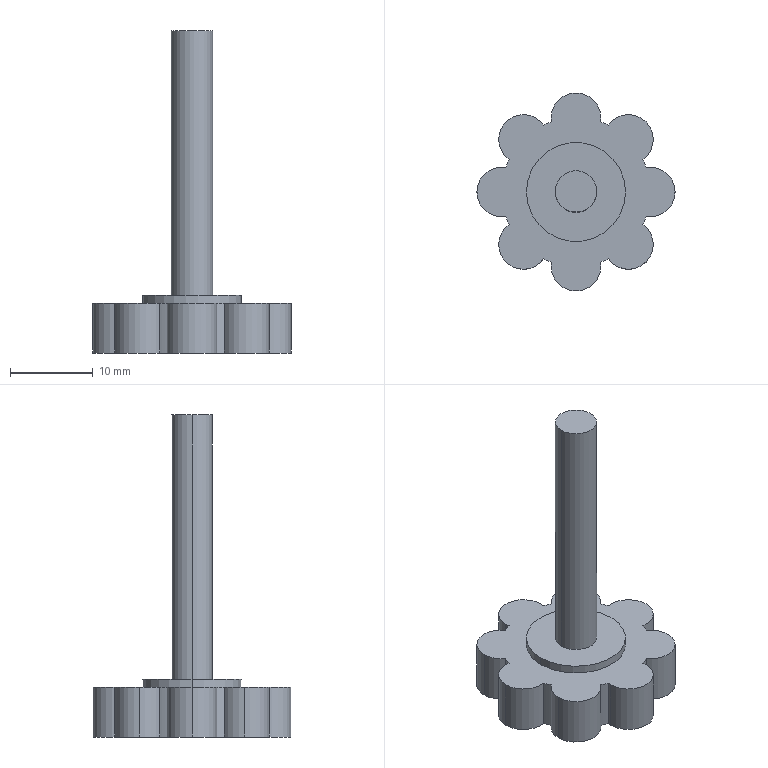Part | SolidWorks | features ICE 3, Extrusion 1 | 1 solid | 34 faces | box 24 x 24 x 39 mm | volume 2986 mm3 | cylinder 29 | plane 5 | commonest cylinder face diameters 6 x15 18 x8 5 x2 7.409 x2 12 x2
STEP:
#1=CARTESIAN_POINT('',(3.705,0.,0.2));
#2=VERTEX_POINT('',#1);
#3=CARTESIAN_POINT('',(-3.705,0.,0.2));
#4=VERTEX_POINT('',#3);
#5=CARTESIAN_POINT('',(0.,0.,0.2));
#6=DIRECTION('',(0.,0.,-1.));
#7=DIRECTION('',(-1.,0.,0.));
#8=AXIS2_PLACEMENT_3D('',#5,#6,#7);
#9=CIRCLE('',#8,3.705);
#10=EDGE_CURVE('',#2,#4,#9,.T.);
#11=ORIENTED_EDGE('',*,*,#10,.F.);
#12=CARTESIAN_POINT('',(3.705,0.,0.));
#13=VERTEX_POINT('',#12);
#14=CARTESIAN_POINT('',(3.705,0.,0.2));
#15=DIRECTION('',(0.,0.,-1.));
#16=VECTOR('',#15,1000.);
#17=LINE('',#14,#16);
#18=EDGE_CURVE('',#2,#13,#17,.T.);
#19=ORIENTED_EDGE('',*,*,#18,.T.);
#20=CARTESIAN_POINT('',(-3.705,0.,0.));
#21=VERTEX_POINT('',#20);
#22=CARTESIAN_POINT('',(0.,0.,0.));
#23=DIRECTION('',(0.,0.,-1.));
#24=DIRECTION('',(-1.,0.,0.));
#25=AXIS2_PLACEMENT_3D('',#22,#23,#24);
#26=CIRCLE('',#25,3.705);
#27=EDGE_CURVE('',#13,#21,#26,.T.);
#28=ORIENTED_EDGE('',*,*,#27,.T.);
#29=CARTESIAN_POINT('',(-3.705,0.,0.2));
#30=DIRECTION('',(0.,0.,-1.));
#31=VECTOR('',#30,1000.);
#32=LINE('',#29,#31);
#33=EDGE_CURVE('',#4,#21,#32,.T.);
#34=ORIENTED_EDGE('',*,*,#33,.F.);
#35=EDGE_LOOP('',(#11,#19,#28,#34));
#36=FACE_OUTER_BOUND('',#35,.T.);
#37=CARTESIAN_POINT('',(0.,0.,0.2));
#38=DIRECTION('',(0.,0.,-1.));
#39=DIRECTION('',(-1.,0.,0.));
#40=AXIS2_PLACEMENT_3D('',#37,#38,#39);
#41=CYLINDRICAL_SURFACE('',#40,3.705);
#42=ADVANCED_FACE('',(#36),#41,.F.);
#43=CARTESIAN_POINT('',(2.5,0.,39.));
#44=VERTEX_POINT('',#43);
#45=CARTESIAN_POINT('',(-2.5,0.,39.));
#46=VERTEX_POINT('',#45);
#47=CARTESIAN_POINT('',(0.,0.,39.));
#48=DIRECTION('',(0.,0.,1.));
#49=DIRECTION('',(1.,0.,0.));
#50=AXIS2_PLACEMENT_3D('',#47,#48,#49);
#51=CIRCLE('',#50,2.5);
#52=EDGE_CURVE('',#44,#46,#51,.T.);
#53=ORIENTED_EDGE('',*,*,#52,.F.);
#54=CARTESIAN_POINT('',(2.5,0.,7.));
#55=VERTEX_POINT('',#54);
#56=CARTESIAN_POINT('',(2.5,0.,39.));
#57=DIRECTION('',(0.,0.,-1.));
#58=VECTOR('',#57,1000.);
#59=LINE('',#56,#58);
#60=EDGE_CURVE('',#44,#55,#59,.T.);
#61=ORIENTED_EDGE('',*,*,#60,.T.);
#62=CARTESIAN_POINT('',(-2.5,0.,7.));
#63=VERTEX_POINT('',#62);
#64=CARTESIAN_POINT('',(0.,0.,7.));
#65=DIRECTION('',(0.,0.,1.));
#66=DIRECTION('',(1.,0.,0.));
#67=AXIS2_PLACEMENT_3D('',#64,#65,#66);
#68=CIRCLE('',#67,2.5);
#69=EDGE_CURVE('',#55,#63,#68,.T.);
#70=ORIENTED_EDGE('',*,*,#69,.T.);
#71=CARTESIAN_POINT('',(-2.5,0.,39.));
#72=DIRECTION('',(0.,0.,-1.));
#73=VECTOR('',#72,1000.);
#74=LINE('',#71,#73);
#75=EDGE_CURVE('',#46,#63,#74,.T.);
#76=ORIENTED_EDGE('',*,*,#75,.F.);
#77=EDGE_LOOP('',(#53,#61,#70,#76));
#78=FACE_OUTER_BOUND('',#77,.T.);
#79=CARTESIAN_POINT('',(0.,0.,39.));
#80=DIRECTION('',(0.,0.,-1.));
#81=DIRECTION('',(-1.,0.,0.));
#82=AXIS2_PLACEMENT_3D('',#79,#80,#81);
#83=CYLINDRICAL_SURFACE('',#82,2.5);
#84=ADVANCED_FACE('',(#78),#83,.T.);
#85=CARTESIAN_POINT('',(6.,0.,7.));
#86=VERTEX_POINT('',#85);
#87=CARTESIAN_POINT('',(-6.,0.,7.));
#88=VERTEX_POINT('',#87);
#89=CARTESIAN_POINT('',(0.,0.,7.));
#90=DIRECTION('',(0.,0.,1.));
#91=DIRECTION('',(1.,0.,0.));
#92=AXIS2_PLACEMENT_3D('',#89,#90,#91);
#93=CIRCLE('',#92,6.);
#94=EDGE_CURVE('',#86,#88,#93,.T.);
#95=ORIENTED_EDGE('',*,*,#94,.F.);
#96=CARTESIAN_POINT('',(6.,0.,6.));
#97=VERTEX_POINT('',#96);
#98=CARTESIAN_POINT('',(6.,0.,7.));
#99=DIRECTION('',(0.,0.,-1.));
#100=VECTOR('',#99,1000.);
#101=LINE('',#98,#100);
#102=EDGE_CURVE('',#86,#97,#101,.T.);
#103=ORIENTED_EDGE('',*,*,#102,.T.);
#104=CARTESIAN_POINT('',(-6.,0.,6.));
#105=VERTEX_POINT('',#104);
#106=CARTESIAN_POINT('',(0.,0.,6.));
#107=DIRECTION('',(0.,0.,-1.));
#108=DIRECTION('',(1.,0.,0.));
#109=AXIS2_PLACEMENT_3D('',#106,#107,#108);
#110=CIRCLE('',#109,6.);
#111=EDGE_CURVE('',#105,#97,#110,.T.);
#112=ORIENTED_EDGE('',*,*,#111,.F.);
#113=CARTESIAN_POINT('',(-6.,0.,7.));
#114=DIRECTION('',(0.,0.,-1.));
#115=VECTOR('',#114,1000.);
#116=LINE('',#113,#115);
#117=EDGE_CURVE('',#88,#105,#116,.T.);
#118=ORIENTED_EDGE('',*,*,#117,.F.);
#119=EDGE_LOOP('',(#95,#103,#112,#118));
#120=FACE_OUTER_BOUND('',#119,.T.);
#121=CARTESIAN_POINT('',(0.,0.,7.));
#122=DIRECTION('',(0.,0.,-1.));
#123=DIRECTION('',(-1.,0.,0.));
#124=AXIS2_PLACEMENT_3D('',#121,#122,#123);
#125=CYLINDRICAL_SURFACE('',#124,6.);
#126=ADVANCED_FACE('',(#120),#125,.T.);
#127=CARTESIAN_POINT('',(-9.364,6.364,6.));
#128=VERTEX_POINT('',#127);
#129=CARTESIAN_POINT('',(-8.102,3.919,6.));
#130=VERTEX_POINT('',#129);
#131=CARTESIAN_POINT('',(-6.364,6.364,6.));
#132=DIRECTION('',(0.,0.,1.));
#133=DIRECTION('',(1.,0.,0.));
#134=AXIS2_PLACEMENT_3D('',#131,#132,#133);
#135=CIRCLE('',#134,3.);
#136=EDGE_CURVE('',#128,#130,#135,.T.);
#137=ORIENTED_EDGE('',*,*,#136,.F.);
#138=CARTESIAN_POINT('',(-9.364,6.364,0.));
#139=VERTEX_POINT('',#138);
#140=CARTESIAN_POINT('',(-9.364,6.364,6.));
#141=DIRECTION('',(0.,0.,-1.));
#142=VECTOR('',#141,1000.);
#143=LINE('',#140,#142);
#144=EDGE_CURVE('',#128,#139,#143,.T.);
#145=ORIENTED_EDGE('',*,*,#144,.T.);
#146=CARTESIAN_POINT('',(-8.102,3.919,0.));
#147=VERTEX_POINT('',#146);
#148=CARTESIAN_POINT('',(-6.364,6.364,0.));
#149=DIRECTION('',(0.,0.,1.));
#150=DIRECTION('',(1.,0.,0.));
#151=AXIS2_PLACEMENT_3D('',#148,#149,#150);
#152=CIRCLE('',#151,3.);
#153=EDGE_CURVE('',#139,#147,#152,.T.);
#154=ORIENTED_EDGE('',*,*,#153,.T.);
#155=CARTESIAN_POINT('',(-8.102,3.919,6.));
#156=DIRECTION('',(0.,0.,-1.));
#157=VECTOR('',#156,1000.);
#158=LINE('',#155,#157);
#159=EDGE_CURVE('',#130,#147,#158,.T.);
#160=ORIENTED_EDGE('',*,*,#159,.F.);
#161=EDGE_LOOP('',(#137,#145,#154,#160));
#162=FACE_OUTER_BOUND('',#161,.T.);
#163=CARTESIAN_POINT('',(-6.364,6.364,6.));
#164=DIRECTION('',(0.,0.,-1.));
#165=DIRECTION('',(-1.,0.,0.));
#166=AXIS2_PLACEMENT_3D('',#163,#164,#165);
#167=CYLINDRICAL_SURFACE('',#166,3.);
#168=ADVANCED_FACE('',(#162),#167,.T.);
#169=CARTESIAN_POINT('',(3.,9.,6.));
#170=VERTEX_POINT('',#169);
#171=CARTESIAN_POINT('',(-3.,9.,6.));
#172=VERTEX_POINT('',#171);
#173=CARTESIAN_POINT('',(0.,9.,6.));
#174=DIRECTION('',(0.,0.,1.));
#175=DIRECTION('',(1.,0.,0.));
#176=AXIS2_PLACEMENT_3D('',#173,#174,#175);
#177=CIRCLE('',#176,3.);
#178=EDGE_CURVE('',#170,#172,#177,.T.);
#179=ORIENTED_EDGE('',*,*,#178,.F.);
#180=CARTESIAN_POINT('',(3.,9.,0.));
#181=VERTEX_POINT('',#180);
#182=CARTESIAN_POINT('',(3.,9.,6.));
#183=DIRECTION('',(0.,0.,-1.));
#184=VECTOR('',#183,1000.);
#185=LINE('',#182,#184);
#186=EDGE_CURVE('',#170,#181,#185,.T.);
#187=ORIENTED_EDGE('',*,*,#186,.T.);
#188=CARTESIAN_POINT('',(-3.,9.,0.));
#189=VERTEX_POINT('',#188);
#190=CARTESIAN_POINT('',(0.,9.,0.));
#191=DIRECTION('',(0.,0.,1.));
#192=DIRECTION('',(1.,0.,0.));
#193=AXIS2_PLACEMENT_3D('',#190,#191,#192);
#194=CIRCLE('',#193,3.);
#195=EDGE_CURVE('',#181,#189,#194,.T.);
#196=ORIENTED_EDGE('',*,*,#195,.T.);
#197=CARTESIAN_POINT('',(-3.,9.,6.));
#198=DIRECTION('',(0.,0.,-1.));
#199=VECTOR('',#198,1000.);
#200=LINE('',#197,#199);
#201=EDGE_CURVE('',#172,#189,#200,.T.);
#202=ORIENTED_EDGE('',*,*,#201,.F.);
#203=EDGE_LOOP('',(#179,#187,#196,#202));
#204=FACE_OUTER_BOUND('',#203,.T.);
#205=CARTESIAN_POINT('',(0.,9.,6.));
#206=DIRECTION('',(0.,0.,-1.));
#207=DIRECTION('',(-1.,0.,0.));
#208=AXIS2_PLACEMENT_3D('',#205,#206,#207);
#209=CYLINDRICAL_SURFACE('',#208,3.);
#210=ADVANCED_FACE('',(#204),#209,.T.);
#211=CARTESIAN_POINT('',(-2.958,8.5,6.));
#212=VERTEX_POINT('',#211);
#213=CARTESIAN_POINT('',(0.,9.,6.));
#214=DIRECTION('',(0.,0.,1.));
#215=DIRECTION('',(1.,0.,0.));
#216=AXIS2_PLACEMENT_3D('',#213,#214,#215);
#217=CIRCLE('',#216,3.);
#218=EDGE_CURVE('',#172,#212,#217,.T.);
#219=ORIENTED_EDGE('',*,*,#218,.F.);
#220=ORIENTED_EDGE('',*,*,#201,.T.);
#221=CARTESIAN_POINT('',(-2.958,8.5,0.));
#222=VERTEX_POINT('',#221);
#223=CARTESIAN_POINT('',(0.,9.,0.));
#224=DIRECTION('',(0.,0.,1.));
#225=DIRECTION('',(1.,0.,0.));
#226=AXIS2_PLACEMENT_3D('',#223,#224,#225);
#227=CIRCLE('',#226,3.);
#228=EDGE_CURVE('',#189,#222,#227,.T.);
#229=ORIENTED_EDGE('',*,*,#228,.T.);
#230=CARTESIAN_POINT('',(-2.958,8.5,6.));
#231=DIRECTION('',(0.,0.,-1.));
#232=VECTOR('',#231,1000.);
#233=LINE('',#230,#232);
#234=EDGE_CURVE('',#212,#222,#233,.T.);
#235=ORIENTED_EDGE('',*,*,#234,.F.);
#236=EDGE_LOOP('',(#219,#220,#229,#235));
#237=FACE_OUTER_BOUND('',#236,.T.);
#238=CARTESIAN_POINT('',(0.,9.,6.));
#239=DIRECTION('',(0.,0.,-1.));
#240=DIRECTION('',(-1.,0.,0.));
#241=AXIS2_PLACEMENT_3D('',#238,#239,#240);
#242=CYLINDRICAL_SURFACE('',#241,3.);
#243=ADVANCED_FACE('',(#237),#242,.T.);
#244=CARTESIAN_POINT('',(3.,-9.,6.));
#245=VERTEX_POINT('',#244);
#246=CARTESIAN_POINT('',(2.958,-8.5,6.));
#247=VERTEX_POINT('',#246);
#248=CARTESIAN_POINT('',(0.,-9.,6.));
#249=DIRECTION('',(0.,0.,1.));
#250=DIRECTION('',(1.,0.,0.));
#251=AXIS2_PLACEMENT_3D('',#248,#249,#250);
#252=CIRCLE('',#251,3.);
#253=EDGE_CURVE('',#245,#247,#252,.T.);
#254=ORIENTED_EDGE('',*,*,#253,.F.);
#255=CARTESIAN_POINT('',(3.,-9.,0.));
#256=VERTEX_POINT('',#255);
#257=CARTESIAN_POINT('',(3.,-9.,6.));
#258=DIRECTION('',(0.,0.,-1.));
#259=VECTOR('',#258,1000.);
#260=LINE('',#257,#259);
#261=EDGE_CURVE('',#245,#256,#260,.T.);
#262=ORIENTED_EDGE('',*,*,#261,.T.);
#263=CARTESIAN_POINT('',(2.958,-8.5,0.));
#264=VERTEX_POINT('',#263);
#265=CARTESIAN_POINT('',(0.,-9.,0.));
#266=DIRECTION('',(0.,0.,1.));
#267=DIRECTION('',(1.,0.,0.));
#268=AXIS2_PLACEMENT_3D('',#265,#266,#267);
#269=CIRCLE('',#268,3.);
#270=EDGE_CURVE('',#256,#264,#269,.T.);
#271=ORIENTED_EDGE('',*,*,#270,.T.);
#272=CARTESIAN_POINT('',(2.958,-8.5,6.));
#273=DIRECTION('',(0.,0.,-1.));
#274=VECTOR('',#273,1000.);
#275=LINE('',#272,#274);
#276=EDGE_CURVE('',#247,#264,#275,.T.);
#277=ORIENTED_EDGE('',*,*,#276,.F.);
#278=EDGE_LOOP('',(#254,#262,#271,#277));
#279=FACE_OUTER_BOUND('',#278,.T.);
#280=CARTESIAN_POINT('',(0.,-9.,6.));
#281=DIRECTION('',(0.,0.,-1.));
#282=DIRECTION('',(-1.,0.,0.));
#283=AXIS2_PLACEMENT_3D('',#280,#281,#282);
#284=CYLINDRICAL_SURFACE('',#283,3.);
#285=ADVANCED_FACE('',(#279),#284,.T.);
#286=ORIENTED_EDGE('',*,*,#261,.F.);
#287=CARTESIAN_POINT('',(-3.,-9.,6.));
#288=VERTEX_POINT('',#287);
#289=CARTESIAN_POINT('',(0.,-9.,6.));
#290=DIRECTION('',(0.,0.,1.));
#291=DIRECTION('',(1.,0.,0.));
#292=AXIS2_PLACEMENT_3D('',#289,#290,#291);
#293=CIRCLE('',#292,3.);
#294=EDGE_CURVE('',#288,#245,#293,.T.);
#295=ORIENTED_EDGE('',*,*,#294,.F.);
#296=CARTESIAN_POINT('',(-3.,-9.,0.));
#297=VERTEX_POINT('',#296);
#298=CARTESIAN_POINT('',(-3.,-9.,6.));
#299=DIRECTION('',(0.,0.,-1.));
#300=VECTOR('',#299,1000.);
#301=LINE('',#298,#300);
#302=EDGE_CURVE('',#288,#297,#301,.T.);
#303=ORIENTED_EDGE('',*,*,#302,.T.);
#304=CARTESIAN_POINT('',(0.,-9.,0.));
#305=DIRECTION('',(0.,0.,1.));
#306=DIRECTION('',(1.,0.,0.));
#307=AXIS2_PLACEMENT_3D('',#304,#305,#306);
#308=CIRCLE('',#307,3.);
#309=EDGE_CURVE('',#297,#256,#308,.T.);
#310=ORIENTED_EDGE('',*,*,#309,.T.);
#311=EDGE_LOOP('',(#286,#295,#303,#310));
#312=FACE_OUTER_BOUND('',#311,.T.);
#313=CARTESIAN_POINT('',(0.,-9.,6.));
#314=DIRECTION('',(0.,0.,-1.));
#315=DIRECTION('',(-1.,0.,0.));
#316=AXIS2_PLACEMENT_3D('',#313,#314,#315);
#317=CYLINDRICAL_SURFACE('',#316,3.);
#318=ADVANCED_FACE('',(#312),#317,.T.);
#319=CARTESIAN_POINT('',(-9.364,-6.364,6.));
#320=VERTEX_POINT('',#319);
#321=CARTESIAN_POINT('',(-3.919,-8.102,6.));
#322=VERTEX_POINT('',#321);
#323=CARTESIAN_POINT('',(-6.364,-6.364,6.));
#324=DIRECTION('',(0.,0.,1.));
#325=DIRECTION('',(1.,0.,0.));
#326=AXIS2_PLACEMENT_3D('',#323,#324,#325);
#327=CIRCLE('',#326,3.);
#328=EDGE_CURVE('',#320,#322,#327,.T.);
#329=ORIENTED_EDGE('',*,*,#328,.F.);
#330=CARTESIAN_POINT('',(-9.364,-6.364,0.));
#331=VERTEX_POINT('',#330);
#332=CARTESIAN_POINT('',(-9.364,-6.364,6.));
#333=DIRECTION('',(0.,0.,-1.));
#334=VECTOR('',#333,1000.);
#335=LINE('',#332,#334);
#336=EDGE_CURVE('',#320,#331,#335,.T.);
#337=ORIENTED_EDGE('',*,*,#336,.T.);
#338=CARTESIAN_POINT('',(-3.919,-8.102,0.));
#339=VERTEX_POINT('',#338);
#340=CARTESIAN_POINT('',(-6.364,-6.364,0.));
#341=DIRECTION('',(0.,0.,1.));
#342=DIRECTION('',(1.,0.,0.));
#343=AXIS2_PLACEMENT_3D('',#340,#341,#342);
#344=CIRCLE('',#343,3.);
#345=EDGE_CURVE('',#331,#339,#344,.T.);
#346=ORIENTED_EDGE('',*,*,#345,.T.);
#347=CARTESIAN_POINT('',(-3.919,-8.102,6.));
#348=DIRECTION('',(0.,0.,-1.));
#349=VECTOR('',#348,1000.);
#350=LINE('',#347,#349);
#351=EDGE_CURVE('',#322,#339,#350,.T.);
#352=ORIENTED_EDGE('',*,*,#351,.F.);
#353=EDGE_LOOP('',(#329,#337,#346,#352));
#354=FACE_OUTER_BOUND('',#353,.T.);
#355=CARTESIAN_POINT('',(-6.364,-6.364,6.));
#356=DIRECTION('',(0.,0.,-1.));
#357=DIRECTION('',(-1.,0.,0.));
#358=AXIS2_PLACEMENT_3D('',#355,#356,#357);
#359=CYLINDRICAL_SURFACE('',#358,3.);
#360=ADVANCED_FACE('',(#354),#359,.T.);
#361=CARTESIAN_POINT('',(-12.,0.,6.));
#362=VERTEX_POINT('',#361);
#363=CARTESIAN_POINT('',(-8.5,-2.958,6.));
#364=VERTEX_POINT('',#363);
#365=CARTESIAN_POINT('',(-9.,0.,6.));
#366=DIRECTION('',(0.,0.,1.));
#367=DIRECTION('',(1.,0.,0.));
#368=AXIS2_PLACEMENT_3D('',#365,#366,#367);
#369=CIRCLE('',#368,3.);
#370=EDGE_CURVE('',#362,#364,#369,.T.);
#371=ORIENTED_EDGE('',*,*,#370,.F.);
#372=CARTESIAN_POINT('',(-12.,0.,0.));
#373=VERTEX_POINT('',#372);
#374=CARTESIAN_POINT('',(-12.,0.,6.));
#375=DIRECTION('',(0.,0.,-1.));
#376=VECTOR('',#375,1000.);
#377=LINE('',#374,#376);
#378=EDGE_CURVE('',#362,#373,#377,.T.);
#379=ORIENTED_EDGE('',*,*,#378,.T.);
#380=CARTESIAN_POINT('',(-8.5,-2.958,0.));
#381=VERTEX_POINT('',#380);
#382=CARTESIAN_POINT('',(-9.,0.,0.));
#383=DIRECTION('',(0.,0.,1.));
#384=DIRECTION('',(1.,0.,0.));
#385=AXIS2_PLACEMENT_3D('',#382,#383,#384);
#386=CIRCLE('',#385,3.);
#387=EDGE_CURVE('',#373,#381,#386,.T.);
#388=ORIENTED_EDGE('',*,*,#387,.T.);
#389=CARTESIAN_POINT('',(-8.5,-2.958,6.));
#390=DIRECTION('',(0.,0.,-1.));
#391=VECTOR('',#390,1000.);
#392=LINE('',#389,#391);
#393=EDGE_CURVE('',#364,#381,#392,.T.);
#394=ORIENTED_EDGE('',*,*,#393,.F.);
#395=EDGE_LOOP('',(#371,#379,#388,#394));
#396=FACE_OUTER_BOUND('',#395,.T.);
#397=CARTESIAN_POINT('',(-9.,0.,6.));
#398=DIRECTION('',(0.,0.,-1.));
#399=DIRECTION('',(-1.,0.,0.));
#400=AXIS2_PLACEMENT_3D('',#397,#398,#399);
#401=CYLINDRICAL_SURFACE('',#400,3.);
#402=ADVANCED_FACE('',(#396),#401,.T.);
#403=CARTESIAN_POINT('',(-8.5,2.958,0.));
#404=VERTEX_POINT('',#403);
#405=CARTESIAN_POINT('',(0.,0.,0.));
#406=DIRECTION('',(0.,0.,1.));
#407=DIRECTION('',(1.,0.,0.));
#408=AXIS2_PLACEMENT_3D('',#405,#406,#407);
#409=CIRCLE('',#408,9.);
#410=EDGE_CURVE('',#147,#404,#409,.T.);
#411=ORIENTED_EDGE('',*,*,#410,.T.);
#412=CARTESIAN_POINT('',(-8.5,2.958,6.));
#413=VERTEX_POINT('',#412);
#414=CARTESIAN_POINT('',(-8.5,2.958,6.));
#415=DIRECTION('',(0.,0.,-1.));
#416=VECTOR('',#415,1000.);
#417=LINE('',#414,#416);
#418=EDGE_CURVE('',#413,#404,#417,.T.);
#419=ORIENTED_EDGE('',*,*,#418,.F.);
#420=CARTESIAN_POINT('',(0.,0.,6.));
#421=DIRECTION('',(0.,0.,1.));
#422=DIRECTION('',(1.,0.,0.));
#423=AXIS2_PLACEMENT_3D('',#420,#421,#422);
#424=CIRCLE('',#423,9.);
#425=EDGE_CURVE('',#130,#413,#424,.T.);
#426=ORIENTED_EDGE('',*,*,#425,.F.);
#427=ORIENTED_EDGE('',*,*,#159,.T.);
#428=EDGE_LOOP('',(#411,#419,#426,#427));
#429=FACE_OUTER_BOUND('',#428,.T.);
#430=CARTESIAN_POINT('',(0.,0.,6.));
#431=DIRECTION('',(0.,0.,-1.));
#432=DIRECTION('',(-1.,0.,0.));
#433=AXIS2_PLACEMENT_3D('',#430,#431,#432);
#434=CYLINDRICAL_SURFACE('',#433,9.);
#435=ADVANCED_FACE('',(#429),#434,.T.);
#436=ORIENTED_EDGE('',*,*,#378,.F.);
#437=CARTESIAN_POINT('',(-9.,0.,6.));
#438=DIRECTION('',(0.,0.,1.));
#439=DIRECTION('',(1.,0.,0.));
#440=AXIS2_PLACEMENT_3D('',#437,#438,#439);
#441=CIRCLE('',#440,3.);
#442=EDGE_CURVE('',#413,#362,#441,.T.);
#443=ORIENTED_EDGE('',*,*,#442,.F.);
#444=ORIENTED_EDGE('',*,*,#418,.T.);
#445=CARTESIAN_POINT('',(-9.,0.,0.));
#446=DIRECTION('',(0.,0.,1.));
#447=DIRECTION('',(1.,0.,0.));
#448=AXIS2_PLACEMENT_3D('',#445,#446,#447);
#449=CIRCLE('',#448,3.);
#450=EDGE_CURVE('',#404,#373,#449,.T.);
#451=ORIENTED_EDGE('',*,*,#450,.T.);
#452=EDGE_LOOP('',(#436,#443,#444,#451));
#453=FACE_OUTER_BOUND('',#452,.T.);
#454=CARTESIAN_POINT('',(-9.,0.,6.));
#455=DIRECTION('',(0.,0.,-1.));
#456=DIRECTION('',(-1.,0.,0.));
#457=AXIS2_PLACEMENT_3D('',#454,#455,#456);
#458=CYLINDRICAL_SURFACE('',#457,3.);
#459=ADVANCED_FACE('',(#453),#458,.T.);
#460=CARTESIAN_POINT('',(-8.102,-3.919,0.));
#461=VERTEX_POINT('',#460);
#462=CARTESIAN_POINT('',(0.,0.,0.));
#463=DIRECTION('',(0.,0.,1.));
#464=DIRECTION('',(1.,0.,0.));
#465=AXIS2_PLACEMENT_3D('',#462,#463,#464);
#466=CIRCLE('',#465,9.);
#467=EDGE_CURVE('',#381,#461,#466,.T.);
#468=ORIENTED_EDGE('',*,*,#467,.T.);
#469=CARTESIAN_POINT('',(-8.102,-3.919,6.));
#470=VERTEX_POINT('',#469);
#471=CARTESIAN_POINT('',(-8.102,-3.919,6.));
#472=DIRECTION('',(0.,0.,-1.));
#473=VECTOR('',#472,1000.);
#474=LINE('',#471,#473);
#475=EDGE_CURVE('',#470,#461,#474,.T.);
#476=ORIENTED_EDGE('',*,*,#475,.F.);
#477=CARTESIAN_POINT('',(0.,0.,6.));
#478=DIRECTION('',(0.,0.,1.));
#479=DIRECTION('',(1.,0.,0.));
#480=AXIS2_PLACEMENT_3D('',#477,#478,#479);
#481=CIRCLE('',#480,9.);
#482=EDGE_CURVE('',#364,#470,#481,.T.);
#483=ORIENTED_EDGE('',*,*,#482,.F.);
#484=ORIENTED_EDGE('',*,*,#393,.T.);
#485=EDGE_LOOP('',(#468,#476,#483,#484));
#486=FACE_OUTER_BOUND('',#485,.T.);
#487=CARTESIAN_POINT('',(0.,0.,6.));
#488=DIRECTION('',(0.,0.,-1.));
#489=DIRECTION('',(-1.,0.,0.));
#490=AXIS2_PLACEMENT_3D('',#487,#488,#489);
#491=CYLINDRICAL_SURFACE('',#490,9.);
#492=ADVANCED_FACE('',(#486),#491,.T.);
#493=ORIENTED_EDGE('',*,*,#336,.F.);
#494=CARTESIAN_POINT('',(-6.364,-6.364,6.));
#495=DIRECTION('',(0.,0.,1.));
#496=DIRECTION('',(1.,0.,0.));
#497=AXIS2_PLACEMENT_3D('',#494,#495,#496);
#498=CIRCLE('',#497,3.);
#499=EDGE_CURVE('',#470,#320,#498,.T.);
#500=ORIENTED_EDGE('',*,*,#499,.F.);
#501=ORIENTED_EDGE('',*,*,#475,.T.);
#502=CARTESIAN_POINT('',(-6.364,-6.364,0.));
#503=DIRECTION('',(0.,0.,1.));
#504=DIRECTION('',(1.,0.,0.));
#505=AXIS2_PLACEMENT_3D('',#502,#503,#504);
#506=CIRCLE('',#505,3.);
#507=EDGE_CURVE('',#461,#331,#506,.T.);
#508=ORIENTED_EDGE('',*,*,#507,.T.);
#509=EDGE_LOOP('',(#493,#500,#501,#508));
#510=FACE_OUTER_BOUND('',#509,.T.);
#511=CARTESIAN_POINT('',(-6.364,-6.364,6.));
#512=DIRECTION('',(0.,0.,-1.));
#513=DIRECTION('',(-1.,0.,0.));
#514=AXIS2_PLACEMENT_3D('',#511,#512,#513);
#515=CYLINDRICAL_SURFACE('',#514,3.);
#516=ADVANCED_FACE('',(#510),#515,.T.);
#517=CARTESIAN_POINT('',(-2.958,-8.5,0.));
#518=VERTEX_POINT('',#517);
#519=CARTESIAN_POINT('',(0.,0.,0.));
#520=DIRECTION('',(0.,0.,1.));
#521=DIRECTION('',(1.,0.,0.));
#522=AXIS2_PLACEMENT_3D('',#519,#520,#521);
#523=CIRCLE('',#522,9.);
#524=EDGE_CURVE('',#339,#518,#523,.T.);
#525=ORIENTED_EDGE('',*,*,#524,.T.);
#526=CARTESIAN_POINT('',(-2.958,-8.5,6.));
#527=VERTEX_POINT('',#526);
#528=CARTESIAN_POINT('',(-2.958,-8.5,6.));
#529=DIRECTION('',(0.,0.,-1.));
#530=VECTOR('',#529,1000.);
#531=LINE('',#528,#530);
#532=EDGE_CURVE('',#527,#518,#531,.T.);
#533=ORIENTED_EDGE('',*,*,#532,.F.);
#534=CARTESIAN_POINT('',(0.,0.,6.));
#535=DIRECTION('',(0.,0.,1.));
#536=DIRECTION('',(1.,0.,0.));
#537=AXIS2_PLACEMENT_3D('',#534,#535,#536);
#538=CIRCLE('',#537,9.);
#539=EDGE_CURVE('',#322,#527,#538,.T.);
#540=ORIENTED_EDGE('',*,*,#539,.F.);
#541=ORIENTED_EDGE('',*,*,#351,.T.);
#542=EDGE_LOOP('',(#525,#533,#540,#541));
#543=FACE_OUTER_BOUND('',#542,.T.);
#544=CARTESIAN_POINT('',(0.,0.,6.));
#545=DIRECTION('',(0.,0.,-1.));
#546=DIRECTION('',(-1.,0.,0.));
#547=AXIS2_PLACEMENT_3D('',#544,#545,#546);
#548=CYLINDRICAL_SURFACE('',#547,9.);
#549=ADVANCED_FACE('',(#543),#548,.T.);
#550=ORIENTED_EDGE('',*,*,#302,.F.);
#551=CARTESIAN_POINT('',(0.,-9.,6.));
#552=DIRECTION('',(0.,0.,1.));
#553=DIRECTION('',(1.,0.,0.));
#554=AXIS2_PLACEMENT_3D('',#551,#552,#553);
#555=CIRCLE('',#554,3.);
#556=EDGE_CURVE('',#527,#288,#555,.T.);
#557=ORIENTED_EDGE('',*,*,#556,.F.);
#558=ORIENTED_EDGE('',*,*,#532,.T.);
#559=CARTESIAN_POINT('',(0.,-9.,0.));
#560=DIRECTION('',(0.,0.,1.));
#561=DIRECTION('',(1.,0.,0.));
#562=AXIS2_PLACEMENT_3D('',#559,#560,#561);
#563=CIRCLE('',#562,3.);
#564=EDGE_CURVE('',#518,#297,#563,.T.);
#565=ORIENTED_EDGE('',*,*,#564,.T.);
#566=EDGE_LOOP('',(#550,#557,#558,#565));
#567=FACE_OUTER_BOUND('',#566,.T.);
#568=CARTESIAN_POINT('',(0.,-9.,6.));
#569=DIRECTION('',(0.,0.,-1.));
#570=DIRECTION('',(-1.,0.,0.));
#571=AXIS2_PLACEMENT_3D('',#568,#569,#570);
#572=CYLINDRICAL_SURFACE('',#571,3.);
#573=ADVANCED_FACE('',(#567),#572,.T.);
#574=CARTESIAN_POINT('',(3.919,-8.102,0.));
#575=VERTEX_POINT('',#574);
#576=CARTESIAN_POINT('',(0.,0.,0.));
#577=DIRECTION('',(0.,0.,1.));
#578=DIRECTION('',(1.,0.,0.));
#579=AXIS2_PLACEMENT_3D('',#576,#577,#578);
#580=CIRCLE('',#579,9.);
#581=EDGE_CURVE('',#264,#575,#580,.T.);
#582=ORIENTED_EDGE('',*,*,#581,.T.);
#583=CARTESIAN_POINT('',(3.919,-8.102,6.));
#584=VERTEX_POINT('',#583);
#585=CARTESIAN_POINT('',(3.919,-8.102,6.));
#586=DIRECTION('',(0.,0.,-1.));
#587=VECTOR('',#586,1000.);
#588=LINE('',#585,#587);
#589=EDGE_CURVE('',#584,#575,#588,.T.);
#590=ORIENTED_EDGE('',*,*,#589,.F.);
#591=CARTESIAN_POINT('',(0.,0.,6.));
#592=DIRECTION('',(0.,0.,1.));
#593=DIRECTION('',(1.,0.,0.));
#594=AXIS2_PLACEMENT_3D('',#591,#592,#593);
#595=CIRCLE('',#594,9.);
#596=EDGE_CURVE('',#247,#584,#595,.T.);
#597=ORIENTED_EDGE('',*,*,#596,.F.);
#598=ORIENTED_EDGE('',*,*,#276,.T.);
#599=EDGE_LOOP('',(#582,#590,#597,#598));
#600=FACE_OUTER_BOUND('',#599,.T.);
#601=CARTESIAN_POINT('',(0.,0.,6.));
#602=DIRECTION('',(0.,0.,-1.));
#603=DIRECTION('',(-1.,0.,0.));
#604=AXIS2_PLACEMENT_3D('',#601,#602,#603);
#605=CYLINDRICAL_SURFACE('',#604,9.);
#606=ADVANCED_FACE('',(#600),#605,.T.);
#607=CARTESIAN_POINT('',(8.102,-3.919,0.));
#608=VERTEX_POINT('',#607);
#609=CARTESIAN_POINT('',(6.364,-6.364,0.));
#610=DIRECTION('',(0.,0.,1.));
#611=DIRECTION('',(1.,0.,0.));
#612=AXIS2_PLACEMENT_3D('',#609,#610,#611);
#613=CIRCLE('',#612,3.);
#614=EDGE_CURVE('',#575,#608,#613,.T.);
#615=ORIENTED_EDGE('',*,*,#614,.T.);
#616=CARTESIAN_POINT('',(8.102,-3.919,6.));
#617=VERTEX_POINT('',#616);
#618=CARTESIAN_POINT('',(8.102,-3.919,6.));
#619=DIRECTION('',(0.,0.,-1.));
#620=VECTOR('',#619,1000.);
#621=LINE('',#618,#620);
#622=EDGE_CURVE('',#617,#608,#621,.T.);
#623=ORIENTED_EDGE('',*,*,#622,.F.);
#624=CARTESIAN_POINT('',(6.364,-6.364,6.));
#625=DIRECTION('',(0.,0.,1.));
#626=DIRECTION('',(1.,0.,0.));
#627=AXIS2_PLACEMENT_3D('',#624,#625,#626);
#628=CIRCLE('',#627,3.);
#629=EDGE_CURVE('',#584,#617,#628,.T.);
#630=ORIENTED_EDGE('',*,*,#629,.F.);
#631=ORIENTED_EDGE('',*,*,#589,.T.);
#632=EDGE_LOOP('',(#615,#623,#630,#631));
#633=FACE_OUTER_BOUND('',#632,.T.);
#634=CARTESIAN_POINT('',(6.364,-6.364,6.));
#635=DIRECTION('',(0.,0.,-1.));
#636=DIRECTION('',(-1.,0.,0.));
#637=AXIS2_PLACEMENT_3D('',#634,#635,#636);
#638=CYLINDRICAL_SURFACE('',#637,3.);
#639=ADVANCED_FACE('',(#633),#638,.T.);
#640=CARTESIAN_POINT('',(8.5,-2.958,0.));
#641=VERTEX_POINT('',#640);
#642=CARTESIAN_POINT('',(0.,0.,0.));
#643=DIRECTION('',(0.,0.,1.));
#644=DIRECTION('',(1.,0.,0.));
#645=AXIS2_PLACEMENT_3D('',#642,#643,#644);
#646=CIRCLE('',#645,9.);
#647=EDGE_CURVE('',#608,#641,#646,.T.);
#648=ORIENTED_EDGE('',*,*,#647,.T.);
#649=CARTESIAN_POINT('',(8.5,-2.958,6.));
#650=VERTEX_POINT('',#649);
#651=CARTESIAN_POINT('',(8.5,-2.958,6.));
#652=DIRECTION('',(0.,0.,-1.));
#653=VECTOR('',#652,1000.);
#654=LINE('',#651,#653);
#655=EDGE_CURVE('',#650,#641,#654,.T.);
#656=ORIENTED_EDGE('',*,*,#655,.F.);
#657=CARTESIAN_POINT('',(0.,0.,6.));
#658=DIRECTION('',(0.,0.,1.));
#659=DIRECTION('',(1.,0.,0.));
#660=AXIS2_PLACEMENT_3D('',#657,#658,#659);
#661=CIRCLE('',#660,9.);
#662=EDGE_CURVE('',#617,#650,#661,.T.);
#663=ORIENTED_EDGE('',*,*,#662,.F.);
#664=ORIENTED_EDGE('',*,*,#622,.T.);
#665=EDGE_LOOP('',(#648,#656,#663,#664));
#666=FACE_OUTER_BOUND('',#665,.T.);
#667=CARTESIAN_POINT('',(0.,0.,6.));
#668=DIRECTION('',(0.,0.,-1.));
#669=DIRECTION('',(-1.,0.,0.));
#670=AXIS2_PLACEMENT_3D('',#667,#668,#669);
#671=CYLINDRICAL_SURFACE('',#670,9.);
#672=ADVANCED_FACE('',(#666),#671,.T.);
#673=CARTESIAN_POINT('',(8.5,2.958,0.));
#674=VERTEX_POINT('',#673);
#675=CARTESIAN_POINT('',(9.,0.,0.));
#676=DIRECTION('',(0.,0.,1.));
#677=DIRECTION('',(1.,0.,0.));
#678=AXIS2_PLACEMENT_3D('',#675,#676,#677);
#679=CIRCLE('',#678,3.);
#680=EDGE_CURVE('',#641,#674,#679,.T.);
#681=ORIENTED_EDGE('',*,*,#680,.T.);
#682=CARTESIAN_POINT('',(8.5,2.958,6.));
#683=VERTEX_POINT('',#682);
#684=CARTESIAN_POINT('',(8.5,2.958,6.));
#685=DIRECTION('',(0.,0.,-1.));
#686=VECTOR('',#685,1000.);
#687=LINE('',#684,#686);
#688=EDGE_CURVE('',#683,#674,#687,.T.);
#689=ORIENTED_EDGE('',*,*,#688,.F.);
#690=CARTESIAN_POINT('',(9.,0.,6.));
#691=DIRECTION('',(0.,0.,1.));
#692=DIRECTION('',(1.,0.,0.));
#693=AXIS2_PLACEMENT_3D('',#690,#691,#692);
#694=CIRCLE('',#693,3.);
#695=EDGE_CURVE('',#650,#683,#694,.T.);
#696=ORIENTED_EDGE('',*,*,#695,.F.);
#697=ORIENTED_EDGE('',*,*,#655,.T.);
#698=EDGE_LOOP('',(#681,#689,#696,#697));
#699=FACE_OUTER_BOUND('',#698,.T.);
#700=CARTESIAN_POINT('',(9.,0.,6.));
#701=DIRECTION('',(0.,0.,-1.));
#702=DIRECTION('',(-1.,0.,0.));
#703=AXIS2_PLACEMENT_3D('',#700,#701,#702);
#704=CYLINDRICAL_SURFACE('',#703,3.);
#705=ADVANCED_FACE('',(#699),#704,.T.);
#706=CARTESIAN_POINT('',(8.102,3.919,0.));
#707=VERTEX_POINT('',#706);
#708=CARTESIAN_POINT('',(0.,0.,0.));
#709=DIRECTION('',(0.,0.,1.));
#710=DIRECTION('',(1.,0.,0.));
#711=AXIS2_PLACEMENT_3D('',#708,#709,#710);
#712=CIRCLE('',#711,9.);
#713=EDGE_CURVE('',#674,#707,#712,.T.);
#714=ORIENTED_EDGE('',*,*,#713,.T.);
#715=CARTESIAN_POINT('',(8.102,3.919,6.));
#716=VERTEX_POINT('',#715);
#717=CARTESIAN_POINT('',(8.102,3.919,6.));
#718=DIRECTION('',(0.,0.,-1.));
#719=VECTOR('',#718,1000.);
#720=LINE('',#717,#719);
#721=EDGE_CURVE('',#716,#707,#720,.T.);
#722=ORIENTED_EDGE('',*,*,#721,.F.);
#723=CARTESIAN_POINT('',(0.,0.,6.));
#724=DIRECTION('',(0.,0.,1.));
#725=DIRECTION('',(1.,0.,0.));
#726=AXIS2_PLACEMENT_3D('',#723,#724,#725);
#727=CIRCLE('',#726,9.);
#728=EDGE_CURVE('',#683,#716,#727,.T.);
#729=ORIENTED_EDGE('',*,*,#728,.F.);
#730=ORIENTED_EDGE('',*,*,#688,.T.);
#731=EDGE_LOOP('',(#714,#722,#729,#730));
#732=FACE_OUTER_BOUND('',#731,.T.);
#733=CARTESIAN_POINT('',(0.,0.,6.));
#734=DIRECTION('',(0.,0.,-1.));
#735=DIRECTION('',(-1.,0.,0.));
#736=AXIS2_PLACEMENT_3D('',#733,#734,#735);
#737=CYLINDRICAL_SURFACE('',#736,9.);
#738=ADVANCED_FACE('',(#732),#737,.T.);
#739=CARTESIAN_POINT('',(3.919,8.102,0.));
#740=VERTEX_POINT('',#739);
#741=CARTESIAN_POINT('',(6.364,6.364,0.));
#742=DIRECTION('',(0.,0.,1.));
#743=DIRECTION('',(1.,0.,0.));
#744=AXIS2_PLACEMENT_3D('',#741,#742,#743);
#745=CIRCLE('',#744,3.);
#746=EDGE_CURVE('',#707,#740,#745,.T.);
#747=ORIENTED_EDGE('',*,*,#746,.T.);
#748=CARTESIAN_POINT('',(3.919,8.102,6.));
#749=VERTEX_POINT('',#748);
#750=CARTESIAN_POINT('',(3.919,8.102,6.));
#751=DIRECTION('',(0.,0.,-1.));
#752=VECTOR('',#751,1000.);
#753=LINE('',#750,#752);
#754=EDGE_CURVE('',#749,#740,#753,.T.);
#755=ORIENTED_EDGE('',*,*,#754,.F.);
#756=CARTESIAN_POINT('',(6.364,6.364,6.));
#757=DIRECTION('',(0.,0.,1.));
#758=DIRECTION('',(1.,0.,0.));
#759=AXIS2_PLACEMENT_3D('',#756,#757,#758);
#760=CIRCLE('',#759,3.);
#761=EDGE_CURVE('',#716,#749,#760,.T.);
#762=ORIENTED_EDGE('',*,*,#761,.F.);
#763=ORIENTED_EDGE('',*,*,#721,.T.);
#764=EDGE_LOOP('',(#747,#755,#762,#763));
#765=FACE_OUTER_BOUND('',#764,.T.);
#766=CARTESIAN_POINT('',(6.364,6.364,6.));
#767=DIRECTION('',(0.,0.,-1.));
#768=DIRECTION('',(-1.,0.,0.));
#769=AXIS2_PLACEMENT_3D('',#766,#767,#768);
#770=CYLINDRICAL_SURFACE('',#769,3.);
#771=ADVANCED_FACE('',(#765),#770,.T.);
#772=CARTESIAN_POINT('',(2.958,8.5,0.));
#773=VERTEX_POINT('',#772);
#774=CARTESIAN_POINT('',(0.,0.,0.));
#775=DIRECTION('',(0.,0.,1.));
#776=DIRECTION('',(1.,0.,0.));
#777=AXIS2_PLACEMENT_3D('',#774,#775,#776);
#778=CIRCLE('',#777,9.);
#779=EDGE_CURVE('',#740,#773,#778,.T.);
#780=ORIENTED_EDGE('',*,*,#779,.T.);
#781=CARTESIAN_POINT('',(2.958,8.5,6.));
#782=VERTEX_POINT('',#781);
#783=CARTESIAN_POINT('',(2.958,8.5,6.));
#784=DIRECTION('',(0.,0.,-1.));
#785=VECTOR('',#784,1000.);
#786=LINE('',#783,#785);
#787=EDGE_CURVE('',#782,#773,#786,.T.);
#788=ORIENTED_EDGE('',*,*,#787,.F.);
#789=CARTESIAN_POINT('',(0.,0.,6.));
#790=DIRECTION('',(0.,0.,1.));
#791=DIRECTION('',(1.,0.,0.));
#792=AXIS2_PLACEMENT_3D('',#789,#790,#791);
#793=CIRCLE('',#792,9.);
#794=EDGE_CURVE('',#749,#782,#793,.T.);
#795=ORIENTED_EDGE('',*,*,#794,.F.);
#796=ORIENTED_EDGE('',*,*,#754,.T.);
#797=EDGE_LOOP('',(#780,#788,#795,#796));
#798=FACE_OUTER_BOUND('',#797,.T.);
#799=CARTESIAN_POINT('',(0.,0.,6.));
#800=DIRECTION('',(0.,0.,-1.));
#801=DIRECTION('',(-1.,0.,0.));
#802=AXIS2_PLACEMENT_3D('',#799,#800,#801);
#803=CYLINDRICAL_SURFACE('',#802,9.);
#804=ADVANCED_FACE('',(#798),#803,.T.);
#805=ORIENTED_EDGE('',*,*,#186,.F.);
#806=CARTESIAN_POINT('',(0.,9.,6.));
#807=DIRECTION('',(0.,0.,1.));
#808=DIRECTION('',(1.,0.,0.));
#809=AXIS2_PLACEMENT_3D('',#806,#807,#808);
#810=CIRCLE('',#809,3.);
#811=EDGE_CURVE('',#782,#170,#810,.T.);
#812=ORIENTED_EDGE('',*,*,#811,.F.);
#813=ORIENTED_EDGE('',*,*,#787,.T.);
#814=CARTESIAN_POINT('',(0.,9.,0.));
#815=DIRECTION('',(0.,0.,1.));
#816=DIRECTION('',(1.,0.,0.));
#817=AXIS2_PLACEMENT_3D('',#814,#815,#816);
#818=CIRCLE('',#817,3.);
#819=EDGE_CURVE('',#773,#181,#818,.T.);
#820=ORIENTED_EDGE('',*,*,#819,.T.);
#821=EDGE_LOOP('',(#805,#812,#813,#820));
#822=FACE_OUTER_BOUND('',#821,.T.);
#823=CARTESIAN_POINT('',(0.,9.,6.));
#824=DIRECTION('',(0.,0.,-1.));
#825=DIRECTION('',(-1.,0.,0.));
#826=AXIS2_PLACEMENT_3D('',#823,#824,#825);
#827=CYLINDRICAL_SURFACE('',#826,3.);
#828=ADVANCED_FACE('',(#822),#827,.T.);
#829=CARTESIAN_POINT('',(-3.919,8.102,0.));
#830=VERTEX_POINT('',#829);
#831=CARTESIAN_POINT('',(0.,0.,0.));
#832=DIRECTION('',(0.,0.,1.));
#833=DIRECTION('',(1.,0.,0.));
#834=AXIS2_PLACEMENT_3D('',#831,#832,#833);
#835=CIRCLE('',#834,9.);
#836=EDGE_CURVE('',#222,#830,#835,.T.);
#837=ORIENTED_EDGE('',*,*,#836,.T.);
#838=CARTESIAN_POINT('',(-3.919,8.102,6.));
#839=VERTEX_POINT('',#838);
#840=CARTESIAN_POINT('',(-3.919,8.102,6.));
#841=DIRECTION('',(0.,0.,-1.));
#842=VECTOR('',#841,1000.);
#843=LINE('',#840,#842);
#844=EDGE_CURVE('',#839,#830,#843,.T.);
#845=ORIENTED_EDGE('',*,*,#844,.F.);
#846=CARTESIAN_POINT('',(0.,0.,6.));
#847=DIRECTION('',(0.,0.,1.));
#848=DIRECTION('',(1.,0.,0.));
#849=AXIS2_PLACEMENT_3D('',#846,#847,#848);
#850=CIRCLE('',#849,9.);
#851=EDGE_CURVE('',#212,#839,#850,.T.);
#852=ORIENTED_EDGE('',*,*,#851,.F.);
#853=ORIENTED_EDGE('',*,*,#234,.T.);
#854=EDGE_LOOP('',(#837,#845,#852,#853));
#855=FACE_OUTER_BOUND('',#854,.T.);
#856=CARTESIAN_POINT('',(0.,0.,6.));
#857=DIRECTION('',(0.,0.,-1.));
#858=DIRECTION('',(-1.,0.,0.));
#859=AXIS2_PLACEMENT_3D('',#856,#857,#858);
#860=CYLINDRICAL_SURFACE('',#859,9.);
#861=ADVANCED_FACE('',(#855),#860,.T.);
#862=ORIENTED_EDGE('',*,*,#144,.F.);
#863=CARTESIAN_POINT('',(-6.364,6.364,6.));
#864=DIRECTION('',(0.,0.,1.));
#865=DIRECTION('',(1.,0.,0.));
#866=AXIS2_PLACEMENT_3D('',#863,#864,#865);
#867=CIRCLE('',#866,3.);
#868=EDGE_CURVE('',#839,#128,#867,.T.);
#869=ORIENTED_EDGE('',*,*,#868,.F.);
#870=ORIENTED_EDGE('',*,*,#844,.T.);
#871=CARTESIAN_POINT('',(-6.364,6.364,0.));
#872=DIRECTION('',(0.,0.,1.));
#873=DIRECTION('',(1.,0.,0.));
#874=AXIS2_PLACEMENT_3D('',#871,#872,#873);
#875=CIRCLE('',#874,3.);
#876=EDGE_CURVE('',#830,#139,#875,.T.);
#877=ORIENTED_EDGE('',*,*,#876,.T.);
#878=EDGE_LOOP('',(#862,#869,#870,#877));
#879=FACE_OUTER_BOUND('',#878,.T.);
#880=CARTESIAN_POINT('',(-6.364,6.364,6.));
#881=DIRECTION('',(0.,0.,-1.));
#882=DIRECTION('',(-1.,0.,0.));
#883=AXIS2_PLACEMENT_3D('',#880,#881,#882);
#884=CYLINDRICAL_SURFACE('',#883,3.);
#885=ADVANCED_FACE('',(#879),#884,.T.);
#886=ORIENTED_EDGE('',*,*,#111,.T.);
#887=CARTESIAN_POINT('',(0.,0.,6.));
#888=DIRECTION('',(0.,0.,-1.));
#889=DIRECTION('',(1.,0.,0.));
#890=AXIS2_PLACEMENT_3D('',#887,#888,#889);
#891=CIRCLE('',#890,6.);
#892=EDGE_CURVE('',#97,#105,#891,.T.);
#893=ORIENTED_EDGE('',*,*,#892,.T.);
#894=EDGE_LOOP('',(#886,#893));
#895=FACE_BOUND('',#894,.T.);
#896=ORIENTED_EDGE('',*,*,#425,.T.);
#897=ORIENTED_EDGE('',*,*,#442,.T.);
#898=ORIENTED_EDGE('',*,*,#370,.T.);
#899=ORIENTED_EDGE('',*,*,#482,.T.);
#900=ORIENTED_EDGE('',*,*,#499,.T.);
#901=ORIENTED_EDGE('',*,*,#328,.T.);
#902=ORIENTED_EDGE('',*,*,#539,.T.);
#903=ORIENTED_EDGE('',*,*,#556,.T.);
#904=ORIENTED_EDGE('',*,*,#294,.T.);
#905=ORIENTED_EDGE('',*,*,#253,.T.);
#906=ORIENTED_EDGE('',*,*,#596,.T.);
#907=ORIENTED_EDGE('',*,*,#629,.T.);
#908=ORIENTED_EDGE('',*,*,#662,.T.);
#909=ORIENTED_EDGE('',*,*,#695,.T.);
#910=ORIENTED_EDGE('',*,*,#728,.T.);
#911=ORIENTED_EDGE('',*,*,#761,.T.);
#912=ORIENTED_EDGE('',*,*,#794,.T.);
#913=ORIENTED_EDGE('',*,*,#811,.T.);
#914=ORIENTED_EDGE('',*,*,#178,.T.);
#915=ORIENTED_EDGE('',*,*,#218,.T.);
#916=ORIENTED_EDGE('',*,*,#851,.T.);
#917=ORIENTED_EDGE('',*,*,#868,.T.);
#918=ORIENTED_EDGE('',*,*,#136,.T.);
#919=EDGE_LOOP('',(#896,#897,#898,#899,#900,#901,#902,#903,#904,#905,#906,#907,#908,#909,#910,#911,#912,#913,#914,#915,#916,#917,#918));
#920=FACE_OUTER_BOUND('',#919,.T.);
#921=CARTESIAN_POINT('',(-4.5,0.,6.));
#922=DIRECTION('',(0.,0.,1.));
#923=DIRECTION('',(1.,0.,0.));
#924=AXIS2_PLACEMENT_3D('',#921,#922,#923);
#925=PLANE('',#924);
#926=ADVANCED_FACE('',(#895,#920),#925,.T.);
#927=CARTESIAN_POINT('',(0.,0.,0.));
#928=DIRECTION('',(0.,0.,-1.));
#929=DIRECTION('',(-1.,0.,0.));
#930=AXIS2_PLACEMENT_3D('',#927,#928,#929);
#931=CIRCLE('',#930,3.705);
#932=EDGE_CURVE('',#21,#13,#931,.T.);
#933=ORIENTED_EDGE('',*,*,#932,.F.);
#934=ORIENTED_EDGE('',*,*,#27,.F.);
#935=EDGE_LOOP('',(#933,#934));
#936=FACE_BOUND('',#935,.T.);
#937=ORIENTED_EDGE('',*,*,#410,.F.);
#938=ORIENTED_EDGE('',*,*,#153,.F.);
#939=ORIENTED_EDGE('',*,*,#876,.F.);
#940=ORIENTED_EDGE('',*,*,#836,.F.);
#941=ORIENTED_EDGE('',*,*,#228,.F.);
#942=ORIENTED_EDGE('',*,*,#195,.F.);
#943=ORIENTED_EDGE('',*,*,#819,.F.);
#944=ORIENTED_EDGE('',*,*,#779,.F.);
#945=ORIENTED_EDGE('',*,*,#746,.F.);
#946=ORIENTED_EDGE('',*,*,#713,.F.);
#947=ORIENTED_EDGE('',*,*,#680,.F.);
#948=ORIENTED_EDGE('',*,*,#647,.F.);
#949=ORIENTED_EDGE('',*,*,#614,.F.);
#950=ORIENTED_EDGE('',*,*,#581,.F.);
#951=ORIENTED_EDGE('',*,*,#270,.F.);
#952=ORIENTED_EDGE('',*,*,#309,.F.);
#953=ORIENTED_EDGE('',*,*,#564,.F.);
#954=ORIENTED_EDGE('',*,*,#524,.F.);
#955=ORIENTED_EDGE('',*,*,#345,.F.);
#956=ORIENTED_EDGE('',*,*,#507,.F.);
#957=ORIENTED_EDGE('',*,*,#467,.F.);
#958=ORIENTED_EDGE('',*,*,#387,.F.);
#959=ORIENTED_EDGE('',*,*,#450,.F.);
#960=EDGE_LOOP('',(#937,#938,#939,#940,#941,#942,#943,#944,#945,#946,#947,#948,#949,#950,#951,#952,#953,#954,#955,#956,#957,#958,#959));
#961=FACE_OUTER_BOUND('',#960,.T.);
#962=CARTESIAN_POINT('',(-4.5,0.,0.));
#963=DIRECTION('',(0.,0.,1.));
#964=DIRECTION('',(1.,0.,0.));
#965=AXIS2_PLACEMENT_3D('',#962,#963,#964);
#966=PLANE('',#965);
#967=ADVANCED_FACE('',(#936,#961),#966,.F.);
#968=ORIENTED_EDGE('',*,*,#102,.F.);
#969=CARTESIAN_POINT('',(0.,0.,7.));
#970=DIRECTION('',(0.,0.,1.));
#971=DIRECTION('',(1.,0.,0.));
#972=AXIS2_PLACEMENT_3D('',#969,#970,#971);
#973=CIRCLE('',#972,6.);
#974=EDGE_CURVE('',#88,#86,#973,.T.);
#975=ORIENTED_EDGE('',*,*,#974,.F.);
#976=ORIENTED_EDGE('',*,*,#117,.T.);
#977=ORIENTED_EDGE('',*,*,#892,.F.);
#978=EDGE_LOOP('',(#968,#975,#976,#977));
#979=FACE_OUTER_BOUND('',#978,.T.);
#980=CARTESIAN_POINT('',(0.,0.,7.));
#981=DIRECTION('',(0.,0.,-1.));
#982=DIRECTION('',(-1.,0.,0.));
#983=AXIS2_PLACEMENT_3D('',#980,#981,#982);
#984=CYLINDRICAL_SURFACE('',#983,6.);
#985=ADVANCED_FACE('',(#979),#984,.T.);
#986=CARTESIAN_POINT('',(0.,0.,7.));
#987=DIRECTION('',(0.,0.,1.));
#988=DIRECTION('',(1.,0.,0.));
#989=AXIS2_PLACEMENT_3D('',#986,#987,#988);
#990=CIRCLE('',#989,2.5);
#991=EDGE_CURVE('',#63,#55,#990,.T.);
#992=ORIENTED_EDGE('',*,*,#991,.F.);
#993=ORIENTED_EDGE('',*,*,#69,.F.);
#994=EDGE_LOOP('',(#992,#993));
#995=FACE_BOUND('',#994,.T.);
#996=ORIENTED_EDGE('',*,*,#974,.T.);
#997=ORIENTED_EDGE('',*,*,#94,.T.);
#998=EDGE_LOOP('',(#996,#997));
#999=FACE_OUTER_BOUND('',#998,.T.);
#1000=CARTESIAN_POINT('',(0.,0.,7.));
#1001=DIRECTION('',(0.,0.,1.));
#1002=DIRECTION('',(1.,0.,0.));
#1003=AXIS2_PLACEMENT_3D('',#1000,#1001,#1002);
#1004=PLANE('',#1003);
#1005=ADVANCED_FACE('',(#995,#999),#1004,.T.);
#1006=CARTESIAN_POINT('',(0.,0.,39.));
#1007=DIRECTION('',(0.,0.,1.));
#1008=DIRECTION('',(1.,0.,0.));
#1009=AXIS2_PLACEMENT_3D('',#1006,#1007,#1008);
#1010=CIRCLE('',#1009,2.5);
#1011=EDGE_CURVE('',#46,#44,#1010,.T.);
#1012=ORIENTED_EDGE('',*,*,#1011,.T.);
#1013=ORIENTED_EDGE('',*,*,#52,.T.);
#1014=EDGE_LOOP('',(#1012,#1013));
#1015=FACE_OUTER_BOUND('',#1014,.T.);
#1016=CARTESIAN_POINT('',(0.,0.,39.));
#1017=DIRECTION('',(0.,0.,1.));
#1018=DIRECTION('',(1.,0.,0.));
#1019=AXIS2_PLACEMENT_3D('',#1016,#1017,#1018);
#1020=PLANE('',#1019);
#1021=ADVANCED_FACE('',(#1015),#1020,.T.);
#1022=ORIENTED_EDGE('',*,*,#60,.F.);
#1023=ORIENTED_EDGE('',*,*,#1011,.F.);
#1024=ORIENTED_EDGE('',*,*,#75,.T.);
#1025=ORIENTED_EDGE('',*,*,#991,.T.);
#1026=EDGE_LOOP('',(#1022,#1023,#1024,#1025));
#1027=FACE_OUTER_BOUND('',#1026,.T.);
#1028=CARTESIAN_POINT('',(0.,0.,39.));
#1029=DIRECTION('',(0.,0.,-1.));
#1030=DIRECTION('',(-1.,0.,0.));
#1031=AXIS2_PLACEMENT_3D('',#1028,#1029,#1030);
#1032=CYLINDRICAL_SURFACE('',#1031,2.5);
#1033=ADVANCED_FACE('',(#1027),#1032,.T.);
#1034=ORIENTED_EDGE('',*,*,#18,.F.);
#1035=CARTESIAN_POINT('',(0.,0.,0.2));
#1036=DIRECTION('',(0.,0.,-1.));
#1037=DIRECTION('',(-1.,0.,0.));
#1038=AXIS2_PLACEMENT_3D('',#1035,#1036,#1037);
#1039=CIRCLE('',#1038,3.705);
#1040=EDGE_CURVE('',#4,#2,#1039,.T.);
#1041=ORIENTED_EDGE('',*,*,#1040,.F.);
#1042=ORIENTED_EDGE('',*,*,#33,.T.);
#1043=ORIENTED_EDGE('',*,*,#932,.T.);
#1044=EDGE_LOOP('',(#1034,#1041,#1042,#1043));
#1045=FACE_OUTER_BOUND('',#1044,.T.);
#1046=CARTESIAN_POINT('',(0.,0.,0.2));
#1047=DIRECTION('',(0.,0.,-1.));
#1048=DIRECTION('',(-1.,0.,0.));
#1049=AXIS2_PLACEMENT_3D('',#1046,#1047,#1048);
#1050=CYLINDRICAL_SURFACE('',#1049,3.705);
#1051=ADVANCED_FACE('',(#1045),#1050,.F.);
#1052=ORIENTED_EDGE('',*,*,#1040,.T.);
#1053=ORIENTED_EDGE('',*,*,#10,.T.);
#1054=EDGE_LOOP('',(#1052,#1053));
#1055=FACE_OUTER_BOUND('',#1054,.T.);
#1056=CARTESIAN_POINT('',(0.,0.,0.2));
#1057=DIRECTION('',(0.,0.,-1.));
#1058=DIRECTION('',(-1.,0.,0.));
#1059=AXIS2_PLACEMENT_3D('',#1056,#1057,#1058);
#1060=PLANE('',#1059);
#1061=ADVANCED_FACE('',(#1055),#1060,.T.);
#1062=CLOSED_SHELL('',(#42,#84,#126,#168,#210,#243,#285,#318,#360,#402,#435,#459,#492,#516,#549,#573,#606,#639,#672,#705,#738,#771,#804,#828,#861,#885,#926,#967,#985,#1005,#1021,#1033,#1051,#1061));
#1063=MANIFOLD_SOLID_BREP('',#1062);
#1064=CARTESIAN_POINT('',(0.,0.,0.));
#1065=DIRECTION('',(0.,0.,1.));
#1066=DIRECTION('',(1.,0.,0.));
#1067=AXIS2_PLACEMENT_3D('',#1064,#1065,#1066);
#1068=(LENGTH_UNIT()NAMED_UNIT(*)SI_UNIT(.MILLI.,.METRE.));
#1069=UNCERTAINTY_MEASURE_WITH_UNIT(LENGTH_MEASURE(0.00001),#1068,'','');
#1070=(NAMED_UNIT(*)PLANE_ANGLE_UNIT()SI_UNIT($,.RADIAN.));
#1071=(NAMED_UNIT(*)SI_UNIT($,.STERADIAN.)SOLID_ANGLE_UNIT());
#1072=(GEOMETRIC_REPRESENTATION_CONTEXT(3)GLOBAL_UNCERTAINTY_ASSIGNED_CONTEXT((#1069))GLOBAL_UNIT_ASSIGNED_CONTEXT((#1068,#1070,#1071))REPRESENTATION_CONTEXT('',''));
#1073=ADVANCED_BREP_SHAPE_REPRESENTATION('',(#1063,#1067),#1072);